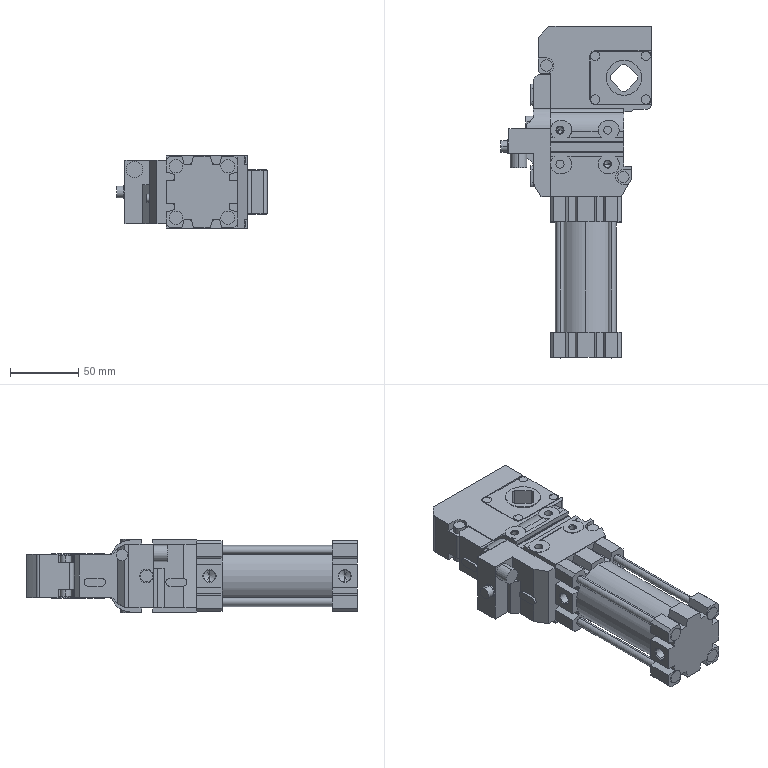Part | STEP file | _CKZT40-X3064L(0)_BODY.stp | 1 solid | 474 faces | box 110.5 x 243.9 x 54 mm | volume 611854 mm3 | plane 278 | cylinder 140 | cone 56 | commonest cylinder face diameters 6 x30 14 x24 4.917 x16 10 x12 8.5 x10 7 x8